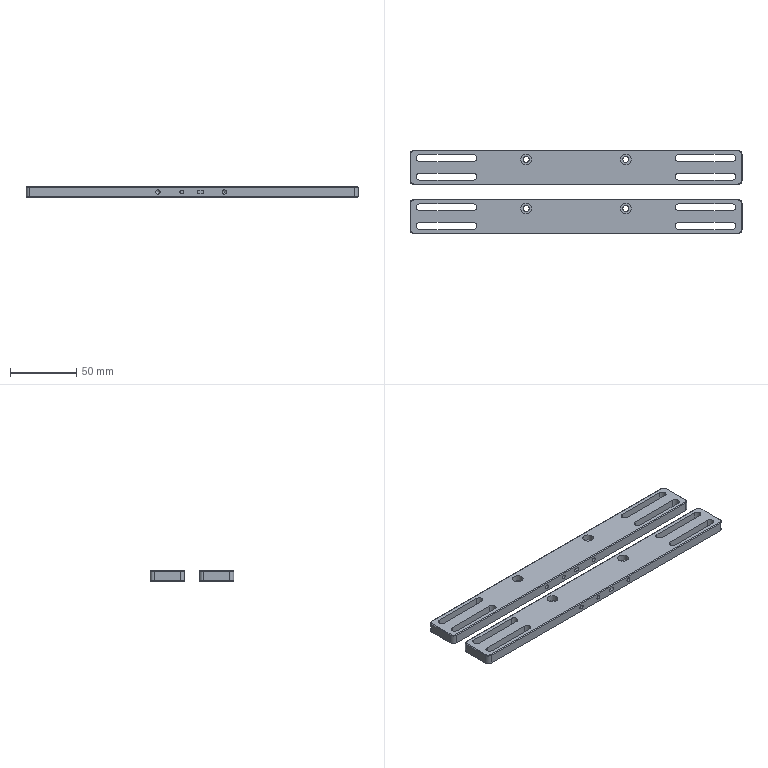NC program | NX | posted with a generic post | part box 250 x 63 x 8 mm
Lines 30 to 910 of 4328:
(ZLEVEL_PROFILE_COPY_COPY , TOOL : D2)
N52 T12 M6
N54 G54
N56 G17 G0 G90 X-7.077 Y0.4 B0. C0. S7500 M3
N58 G43 Z30. H12
N60 Z0.5
N62 G94 G1 X-7.191 Z0.494 F1000.
N64 X-7.207 Y0.396 Z0.493
N66 X-7.366 Y0.312 Z0.484
N68 X-7.496 Y0.108 Z0.471
N70 X-7.488 Y-0.134 Z0.458
N72 X-7.394 Y-0.287 Z0.449
N74 X-7.191 Y-0.4 Z0.437
N76 X-5.511 Z0.349
N78 X-5.323 Y-0.301 Z0.338
N80 X-5.209 Y-0.122 Z0.326
N82 X-5.195 Y0.057 Z0.317
N84 X-5.299 Y0.278 Z0.304
N86 X-5.511 Y0.4 Z0.291
N88 X-7.191 Z0.203
N90 X-7.207 Y0.396
N92 X-7.366 Y0.312 Z0.193
N94 X-7.496 Y0.108 Z0.18
N96 X-7.488 Y-0.134 Z0.168
N98 X-7.394 Y-0.287 Z0.158
N100 X-7.191 Y-0.4 Z0.146
N102 X-5.511 Z0.058
N104 X-5.323 Y-0.301 Z0.047
N106 X-5.209 Y-0.122 Z0.036
N108 X-5.195 Y0.057 Z0.026
N110 X-5.299 Y0.278 Z0.014
N112 X-5.511 Y0.4 Z0.001
N114 X-7.191 Z-0.087
N116 X-7.207 Y0.396 Z-0.088
N118 X-7.366 Y0.312 Z-0.098
N120 X-7.496 Y0.108 Z-0.11
N122 X-7.488 Y-0.134 Z-0.123
N124 X-7.394 Y-0.287 Z-0.132
N126 X-7.191 Y-0.4 Z-0.145
N128 X-7.101 Z-0.149
N130 X-5.601
N132 G3 X-5.201 Y0. R0.4
N134 X-5.601 Y0.4 R0.4
N136 G1 X-7.101
N138 G3 X-7.501 Y0. R0.4
N140 X-7.101 Y-0.4 R0.4
N142 G1 X-5.757 Z-0.198
N144 X-5.654 Y-0.399 Z-0.201
N146 X-5.555 Y-0.389 Z-0.205
N148 X-5.506 Y-0.381 Z-0.207
N150 X-5.454 Y-0.363 Z-0.209
N152 X-5.378 Y-0.321 Z-0.212
N154 X-5.344 Y-0.296 Z-0.214
N156 X-5.292 Y-0.244 Z-0.216
N158 X-5.251 Y-0.179 Z-0.219
N160 X-5.227 Y-0.116 Z-0.222
N162 X-5.214 Y-0.059 Z-0.224
N164 X-5.21 Y0.023 Z-0.227
N166 X-5.218 Y0.089 Z-0.229
N168 X-5.235 Y0.14 Z-0.231
N170 X-5.276 Y0.218 Z-0.235
N172 X-5.301 Y0.253 Z-0.236
N174 X-5.351 Y0.303 Z-0.239
N176 X-5.408 Y0.34 Z-0.241
N178 X-5.437 Y0.357 Z-0.243
N180 X-5.469 Y0.368 Z-0.244
N182 X-5.534 Y0.386 Z-0.246
N184 X-5.636 Y0.397 Z-0.25
N186 X-5.739 Y0.4 Z-0.254
N188 X-6.979 Z-0.299
N190 X-7.101
N192 G3 X-7.501 Y0. R0.4
N194 X-7.101 Y-0.4 R0.4
N196 G1 X-5.757 Z-0.347
N198 X-5.654 Y-0.399 Z-0.351
N200 X-5.555 Y-0.389 Z-0.354
N202 X-5.506 Y-0.381 Z-0.356
N204 X-5.454 Y-0.363 Z-0.358
N206 X-5.378 Y-0.321 Z-0.361
N208 X-5.344 Y-0.296 Z-0.363
N210 X-5.292 Y-0.244 Z-0.366
N212 X-5.251 Y-0.179 Z-0.368
N214 X-5.227 Y-0.116 Z-0.371
N216 X-5.214 Y-0.059 Z-0.373
N218 X-5.21 Y0.023 Z-0.376
N220 X-5.218 Y0.089 Z-0.379
N222 X-5.235 Y0.139 Z-0.381
N224 X-5.276 Y0.218 Z-0.384
N226 X-5.301 Y0.253 Z-0.385
N228 X-5.351 Y0.303 Z-0.388
N230 X-5.408 Y0.34 Z-0.391
N232 X-5.437 Y0.357 Z-0.392
N234 X-5.468 Y0.368 Z-0.393
N236 X-5.534 Y0.386 Z-0.396
N238 X-5.636 Y0.397 Z-0.399
N240 X-5.739 Y0.4 Z-0.403
N242 X-6.979 Z-0.448
N244 X-7.101
N246 G3 X-7.501 Y0. R0.4
N248 X-7.101 Y-0.4 R0.4
N250 G1 X-5.757 Z-0.496
N252 X-5.654 Y-0.399 Z-0.5
N254 X-5.555 Y-0.389 Z-0.504
N256 X-5.506 Y-0.381 Z-0.505
N258 X-5.454 Y-0.363 Z-0.507
N260 X-5.377 Y-0.322 Z-0.511
N262 X-5.344 Y-0.296 Z-0.512
N264 X-5.292 Y-0.244 Z-0.515
N266 X-5.251 Y-0.179 Z-0.518
N268 X-5.227 Y-0.116 Z-0.52
N270 X-5.214 Y-0.059 Z-0.522
N272 X-5.21 Y0.023 Z-0.525
N274 X-5.217 Y0.089 Z-0.528
N276 X-5.235 Y0.139 Z-0.53
N278 X-5.277 Y0.219 Z-0.533
N280 X-5.302 Y0.255 Z-0.535
N282 X-5.351 Y0.303 Z-0.537
N284 X-5.408 Y0.34 Z-0.54
N286 X-5.437 Y0.357 Z-0.541
N288 X-5.469 Y0.368 Z-0.542
N290 X-5.534 Y0.386 Z-0.545
N292 X-5.636 Y0.397 Z-0.549
N294 X-5.739 Y0.4 Z-0.552
N296 X-6.979 Z-0.597
N298 X-7.101
N300 G3 X-7.501 Y0. R0.4
N302 X-7.101 Y-0.4 R0.4
N304 G1 X-5.757 Z-0.646
N306 X-5.654 Y-0.399 Z-0.649
N308 X-5.555 Y-0.388 Z-0.653
N310 X-5.506 Y-0.381 Z-0.655
N312 X-5.454 Y-0.363 Z-0.657
N314 X-5.377 Y-0.322 Z-0.66
N316 X-5.344 Y-0.296 Z-0.661
N318 X-5.292 Y-0.244 Z-0.664
N320 X-5.251 Y-0.179 Z-0.667
N322 X-5.227 Y-0.116 Z-0.669
N324 X-5.214 Y-0.059 Z-0.672
N326 X-5.21 Y0.023 Z-0.675
N328 X-5.217 Y0.089 Z-0.677
N330 X-5.235 Y0.139 Z-0.679
N332 X-5.277 Y0.219 Z-0.682
N334 X-5.302 Y0.255 Z-0.684
N336 X-5.351 Y0.303 Z-0.687
N338 X-5.408 Y0.34 Z-0.689
N340 X-5.437 Y0.357 Z-0.69
N342 X-5.469 Y0.368 Z-0.692
N344 X-5.534 Y0.386 Z-0.694
N346 X-5.636 Y0.397 Z-0.698
N348 X-5.739 Y0.4 Z-0.701
N350 X-6.979 Z-0.746
N352 X-7.101
N354 G3 X-7.501 Y0. R0.4
N356 X-7.101 Y-0.4 R0.4
N358 G1 X-5.757 Z-0.795
N360 X-5.654 Y-0.399 Z-0.799
N362 X-5.555 Y-0.388 Z-0.802
N364 X-5.506 Y-0.381 Z-0.804
N366 X-5.454 Y-0.363 Z-0.806
N368 X-5.377 Y-0.322 Z-0.809
N370 X-5.344 Y-0.296 Z-0.811
N372 X-5.292 Y-0.244 Z-0.813
N374 X-5.251 Y-0.178 Z-0.816
N376 X-5.236 Y-0.143 Z-0.818
N378 X-5.227 Y-0.116 Z-0.819
N380 X-5.214 Y-0.059 Z-0.821
N382 X-5.21 Y0.023 Z-0.824
N384 X-5.217 Y0.09 Z-0.826
N386 X-5.235 Y0.139 Z-0.828
N388 X-5.277 Y0.219 Z-0.832
N390 X-5.302 Y0.255 Z-0.833
N392 X-5.351 Y0.303 Z-0.836
N394 X-5.408 Y0.34 Z-0.838
N396 X-5.437 Y0.357 Z-0.84
N398 X-5.469 Y0.368 Z-0.841
N400 X-5.534 Y0.386 Z-0.843
N402 X-5.636 Y0.397 Z-0.847
N404 X-5.739 Y0.4 Z-0.851
N406 X-6.979 Z-0.896
N408 X-7.101
N410 G3 X-7.501 Y0. R0.4
N412 X-7.101 Y-0.4 R0.4
N414 G1 X-5.757 Z-0.944
N416 X-5.654 Y-0.399 Z-0.948
N418 X-5.555 Y-0.388 Z-0.951
N420 X-5.506 Y-0.381 Z-0.953
N422 X-5.454 Y-0.363 Z-0.955
N424 X-5.377 Y-0.322 Z-0.958
N426 X-5.344 Y-0.296 Z-0.96
N428 X-5.292 Y-0.244 Z-0.963
N430 X-5.251 Y-0.178 Z-0.966
N432 X-5.236 Y-0.143 Z-0.967
N434 X-5.227 Y-0.116 Z-0.968
N436 X-5.214 Y-0.059 Z-0.97
N438 X-5.21 Y0.023 Z-0.973
N440 X-5.217 Y0.089 Z-0.976
N442 X-5.235 Y0.139 Z-0.978
N444 X-5.277 Y0.219 Z-0.981
N446 X-5.302 Y0.255 Z-0.983
N448 X-5.351 Y0.303 Z-0.985
N450 X-5.408 Y0.34 Z-0.988
N452 X-5.437 Y0.357 Z-0.989
N454 X-5.469 Y0.368 Z-0.99
N456 X-5.534 Y0.386 Z-0.993
N458 X-5.636 Y0.397 Z-0.996
N460 X-5.739 Y0.4 Z-1.
N462 X-6.979 Z-1.045
N464 X-7.101
N466 G3 X-7.501 Y0. R0.4
N468 X-7.101 Y-0.4 R0.4
N470 G1 X-5.757 Z-1.093
N472 X-5.654 Y-0.399 Z-1.097
N474 X-5.555 Y-0.388 Z-1.101
N476 X-5.506 Y-0.381 Z-1.102
N478 X-5.454 Y-0.363 Z-1.104
N480 X-5.377 Y-0.322 Z-1.108
N482 X-5.344 Y-0.296 Z-1.109
N484 X-5.292 Y-0.244 Z-1.112
N486 X-5.251 Y-0.178 Z-1.115
N488 X-5.236 Y-0.143 Z-1.116
N490 X-5.227 Y-0.116 Z-1.117
N492 X-5.214 Y-0.059 Z-1.119
N494 X-5.21 Y0.023 Z-1.122
N496 X-5.217 Y0.089 Z-1.125
N498 X-5.235 Y0.139 Z-1.127
N500 X-5.277 Y0.219 Z-1.13
N502 X-5.302 Y0.255 Z-1.132
N504 X-5.351 Y0.303 Z-1.134
N506 X-5.408 Y0.34 Z-1.137
N508 X-5.437 Y0.357 Z-1.138
N510 X-5.469 Y0.368 Z-1.139
N512 X-5.534 Y0.386 Z-1.142
N514 X-5.636 Y0.397 Z-1.146
N516 X-5.739 Y0.4 Z-1.149
N518 X-6.979 Z-1.194
N520 X-7.101
N522 G3 X-7.501 Y0. R0.4
N524 X-7.101 Y-0.4 R0.4
N526 G1 X-5.757 Z-1.243
N528 X-5.654 Y-0.399 Z-1.246
N530 X-5.555 Y-0.388 Z-1.25
N532 X-5.506 Y-0.381 Z-1.252
N534 X-5.454 Y-0.363 Z-1.254
N536 X-5.377 Y-0.322 Z-1.257
N538 X-5.344 Y-0.296 Z-1.258
N540 X-5.292 Y-0.244 Z-1.261
N542 X-5.251 Y-0.178 Z-1.264
N544 X-5.236 Y-0.143 Z-1.265
N546 X-5.227 Y-0.116 Z-1.267
N548 X-5.214 Y-0.059 Z-1.269
N550 X-5.21 Y0.023 Z-1.272
N552 X-5.217 Y0.089 Z-1.274
N554 X-5.236 Y0.139 Z-1.276
N556 X-5.277 Y0.219 Z-1.279
N558 X-5.302 Y0.255 Z-1.281
N560 X-5.351 Y0.303 Z-1.284
N562 X-5.408 Y0.34 Z-1.286
N564 X-5.437 Y0.357 Z-1.287
N566 X-5.469 Y0.368 Z-1.289
N568 X-5.534 Y0.386 Z-1.291
N570 X-5.636 Y0.397 Z-1.295
N572 X-5.739 Y0.4 Z-1.299
N574 X-6.979 Z-1.343
N576 X-7.101
N578 G3 X-7.501 Y0. R0.4
N580 X-7.101 Y-0.4 R0.4
N582 G1 X-5.757 Z-1.392
N584 X-5.654 Y-0.399 Z-1.396
N586 X-5.555 Y-0.388 Z-1.399
N588 X-5.506 Y-0.381 Z-1.401
N590 X-5.454 Y-0.363 Z-1.403
N592 X-5.377 Y-0.322 Z-1.406
N594 X-5.344 Y-0.296 Z-1.408
N596 X-5.292 Y-0.244 Z-1.41
N598 X-5.251 Y-0.178 Z-1.413
N600 X-5.236 Y-0.143 Z-1.415
N602 X-5.227 Y-0.116 Z-1.416
N604 X-5.214 Y-0.059 Z-1.418
N606 X-5.21 Y0.023 Z-1.421
N608 X-5.218 Y0.089 Z-1.423
N610 X-5.236 Y0.139 Z-1.425
N612 X-5.276 Y0.219 Z-1.429
N614 X-5.302 Y0.255 Z-1.43
N616 X-5.351 Y0.303 Z-1.433
N618 X-5.408 Y0.34 Z-1.435
N620 X-5.437 Y0.357 Z-1.437
N622 X-5.469 Y0.368 Z-1.438
N624 X-5.534 Y0.386 Z-1.44
N626 X-5.636 Y0.397 Z-1.444
N628 X-5.739 Y0.4 Z-1.448
N630 X-6.979 Z-1.493
N632 X-7.101
N634 G3 X-7.501 Y0. R0.4
N636 X-7.101 Y-0.4 R0.4
N638 G1 X-5.757 Z-1.541
N640 X-5.654 Y-0.399 Z-1.545
N642 X-5.555 Y-0.388 Z-1.548
N644 X-5.506 Y-0.381 Z-1.55
N646 X-5.454 Y-0.363 Z-1.552
N648 X-5.377 Y-0.322 Z-1.555
N650 X-5.344 Y-0.296 Z-1.557
N652 X-5.292 Y-0.244 Z-1.56
N654 X-5.251 Y-0.178 Z-1.563
N656 X-5.236 Y-0.143 Z-1.564
N658 X-5.227 Y-0.116 Z-1.565
N660 X-5.214 Y-0.059 Z-1.567
N662 X-5.21 Y0.023 Z-1.57
N664 X-5.218 Y0.089 Z-1.573
N666 X-5.236 Y0.139 Z-1.575
N668 X-5.276 Y0.219 Z-1.578
N670 X-5.302 Y0.255 Z-1.58
N672 X-5.351 Y0.303 Z-1.582
N674 X-5.408 Y0.34 Z-1.585
N676 X-5.437 Y0.357 Z-1.586
N678 X-5.469 Y0.368 Z-1.587
N680 X-5.534 Y0.386 Z-1.59
N682 X-5.636 Y0.397 Z-1.593
N684 X-5.739 Y0.4 Z-1.597
N686 X-6.979 Z-1.642
N688 X-7.101
N690 G3 X-7.501 Y0. R0.4
N692 X-7.101 Y-0.4 R0.4
N694 G1 X-5.757 Z-1.69
N696 X-5.654 Y-0.399 Z-1.694
N698 X-5.555 Y-0.388 Z-1.698
N700 X-5.506 Y-0.381 Z-1.699
N702 X-5.454 Y-0.363 Z-1.701
N704 X-5.377 Y-0.322 Z-1.705
N706 X-5.344 Y-0.296 Z-1.706
N708 X-5.292 Y-0.244 Z-1.709
N710 X-5.251 Y-0.178 Z-1.712
N712 X-5.237 Y-0.143 Z-1.713
N714 X-5.227 Y-0.116 Z-1.714
N716 X-5.214 Y-0.059 Z-1.716
N718 X-5.21 Y0.023 Z-1.719
N720 X-5.218 Y0.089 Z-1.722
N722 X-5.236 Y0.139 Z-1.724
N724 X-5.276 Y0.219 Z-1.727
N726 X-5.302 Y0.254 Z-1.729
N728 X-5.351 Y0.303 Z-1.731
N730 X-5.408 Y0.34 Z-1.734
N732 X-5.437 Y0.357 Z-1.735
N734 X-5.469 Y0.368 Z-1.736
N736 X-5.534 Y0.386 Z-1.739
N738 X-5.636 Y0.397 Z-1.743
N740 X-5.739 Y0.4 Z-1.746
N742 X-6.979 Z-1.791
N744 X-7.101
N746 G3 X-7.501 Y0. R0.4
N748 X-7.101 Y-0.4 R0.4
N750 G1 X-5.757 Z-1.84
N752 X-5.654 Y-0.399 Z-1.843
N754 X-5.555 Y-0.388 Z-1.847
N756 X-5.506 Y-0.381 Z-1.849
N758 X-5.454 Y-0.363 Z-1.851
N760 X-5.377 Y-0.322 Z-1.854
N762 X-5.344 Y-0.296 Z-1.855
N764 X-5.292 Y-0.244 Z-1.858
N766 X-5.251 Y-0.178 Z-1.861
N768 X-5.237 Y-0.143 Z-1.862
N770 X-5.227 Y-0.116 Z-1.864
N772 X-5.214 Y-0.059 Z-1.866
N774 X-5.21 Y0.023 Z-1.869
N776 X-5.218 Y0.089 Z-1.871
N778 X-5.236 Y0.139 Z-1.873
N780 X-5.276 Y0.219 Z-1.876
N782 X-5.302 Y0.254 Z-1.878
N784 X-5.351 Y0.303 Z-1.881
N786 X-5.408 Y0.34 Z-1.883
N788 X-5.437 Y0.357 Z-1.884
N790 X-5.469 Y0.368 Z-1.886
N792 X-5.534 Y0.386 Z-1.888
N794 X-5.636 Y0.397 Z-1.892
N796 X-5.739 Y0.4 Z-1.896
N798 X-6.979 Z-1.94
N800 X-7.101
N802 G3 X-7.501 Y0. R0.4
N804 X-7.101 Y-0.4 R0.4
N806 G1 X-5.757 Z-1.989
N808 X-5.654 Y-0.399 Z-1.993
N810 X-5.555 Y-0.388 Z-1.996
N812 X-5.506 Y-0.381 Z-1.998
N814 X-5.454 Y-0.363 Z-2.
N816 X-5.378 Y-0.322 Z-2.003
N818 X-5.344 Y-0.296 Z-2.005
N820 X-5.292 Y-0.244 Z-2.007
N822 X-5.251 Y-0.178 Z-2.01
N824 X-5.237 Y-0.143 Z-2.012
N826 X-5.227 Y-0.116 Z-2.013
N828 X-5.214 Y-0.059 Z-2.015
N830 X-5.21 Y0.023 Z-2.018
N832 X-5.218 Y0.089 Z-2.02
N834 X-5.236 Y0.139 Z-2.022
N836 X-5.276 Y0.219 Z-2.026
N838 X-5.302 Y0.254 Z-2.027
N840 X-5.351 Y0.303 Z-2.03
N842 X-5.408 Y0.34 Z-2.032
N844 X-5.437 Y0.357 Z-2.034
N846 X-5.469 Y0.368 Z-2.035
N848 X-5.534 Y0.386 Z-2.037
N850 X-5.636 Y0.397 Z-2.041
N852 X-5.739 Y0.4 Z-2.045
N854 X-6.979 Z-2.09
N856 X-7.101
N858 G3 X-7.501 Y0. R0.4
N860 X-7.101 Y-0.4 R0.4
N862 G1 X-5.757 Z-2.138
N864 X-5.654 Y-0.399 Z-2.142
N866 X-5.555 Y-0.388 Z-2.145
N868 X-5.506 Y-0.381 Z-2.147
N870 X-5.454 Y-0.363 Z-2.149
N872 X-5.378 Y-0.322 Z-2.152
N874 X-5.344 Y-0.296 Z-2.154
N876 X-5.292 Y-0.244 Z-2.157
N878 X-5.251 Y-0.178 Z-2.16
N880 X-5.237 Y-0.143 Z-2.161
N882 X-5.227 Y-0.116 Z-2.162
N884 X-5.214 Y-0.059 Z-2.164
N886 X-5.21 Y0.023 Z-2.167
N888 X-5.218 Y0.089 Z-2.17
N890 X-5.236 Y0.139 Z-2.172
N892 X-5.276 Y0.219 Z-2.175
N894 X-5.302 Y0.254 Z-2.177
N896 X-5.351 Y0.303 Z-2.179
N898 X-5.408 Y0.34 Z-2.182
N900 X-5.437 Y0.357 Z-2.183
N902 X-5.469 Y0.368 Z-2.184
N904 X-5.534 Y0.386 Z-2.187
N906 X-5.636 Y0.397 Z-2.19
N908 X-5.739 Y0.4 Z-2.194
N910 X-6.979 Z-2.239
N912 X-7.101
N914 G3 X-7.501 Y0. R0.4
N916 X-7.101 Y-0.4 R0.4
N918 G1 X-5.757 Z-2.287
N920 X-5.654 Y-0.399 Z-2.291
N922 X-5.555 Y-0.388 Z-2.295
N924 X-5.506 Y-0.381 Z-2.296
N926 X-5.454 Y-0.363 Z-2.299
N928 X-5.378 Y-0.322 Z-2.302
N930 X-5.344 Y-0.296 Z-2.303
N932 X-5.292 Y-0.244 Z-2.306
N934 X-5.251 Y-0.178 Z-2.309
N936 X-5.237 Y-0.143 Z-2.31
N938 X-5.227 Y-0.116 Z-2.311
N940 X-5.214 Y-0.059 Z-2.313
N942 X-5.21 Y0.023 Z-2.316
N944 X-5.218 Y0.089 Z-2.319
N946 X-5.236 Y0.139 Z-2.321
N948 X-5.276 Y0.219 Z-2.324
N950 X-5.302 Y0.254 Z-2.326
N952 X-5.351 Y0.303 Z-2.328
N954 X-5.408 Y0.34 Z-2.331
N956 X-5.437 Y0.357 Z-2.332
N958 X-5.468 Y0.368 Z-2.333
N960 X-5.534 Y0.386 Z-2.336
N962 X-5.636 Y0.397 Z-2.34
N964 X-5.739 Y0.4 Z-2.343
N966 X-6.979 Z-2.388
N968 X-7.101
N970 G3 X-7.501 Y0. R0.4
N972 X-7.101 Y-0.4 R0.4
N974 G1 X-5.757 Z-2.437
N976 X-5.654 Y-0.399 Z-2.44
N978 X-5.555 Y-0.388 Z-2.444
N980 X-5.506 Y-0.381 Z-2.446
N982 X-5.454 Y-0.363 Z-2.448
N984 X-5.378 Y-0.322 Z-2.451
N986 X-5.344 Y-0.296 Z-2.452
N988 X-5.292 Y-0.244 Z-2.455
N990 X-5.251 Y-0.178 Z-2.458
N992 X-5.237 Y-0.143 Z-2.459
N994 X-5.227 Y-0.116 Z-2.461
N996 X-5.214 Y-0.059 Z-2.463
N998 X-5.21 Y0.023 Z-2.466
N1000 X-5.218 Y0.089 Z-2.468
N1002 X-5.236 Y0.139 Z-2.47
N1004 X-5.276 Y0.219 Z-2.473
N1006 X-5.302 Y0.254 Z-2.475
N1008 X-5.351 Y0.303 Z-2.478
N1010 X-5.408 Y0.34 Z-2.48
N1012 X-5.437 Y0.357 Z-2.481
N1014 X-5.468 Y0.368 Z-2.483
N1016 X-5.534 Y0.386 Z-2.485
N1018 X-5.636 Y0.397 Z-2.489
N1020 X-5.739 Y0.4 Z-2.493
N1022 X-6.979 Z-2.537
N1024 X-7.101
N1026 G3 X-7.501 Y0. R0.4
N1028 X-7.101 Y-0.4 R0.4
N1030 G1 X-5.757 Z-2.586
N1032 X-5.654 Y-0.399 Z-2.59
N1034 X-5.555 Y-0.388 Z-2.593
N1036 X-5.506 Y-0.381 Z-2.595
N1038 X-5.454 Y-0.363 Z-2.597
N1040 X-5.378 Y-0.322 Z-2.6
N1042 X-5.344 Y-0.296 Z-2.602
N1044 X-5.292 Y-0.244 Z-2.604
N1046 X-5.252 Y-0.178 Z-2.607
N1048 X-5.237 Y-0.143 Z-2.609
N1050 X-5.227 Y-0.116 Z-2.61
N1052 X-5.214 Y-0.059 Z-2.612
N1054 X-5.21 Y0.023 Z-2.615
N1056 X-5.218 Y0.089 Z-2.617
N1058 X-5.236 Y0.139 Z-2.619
N1060 X-5.276 Y0.219 Z-2.623
N1062 X-5.302 Y0.254 Z-2.624
N1064 X-5.351 Y0.303 Z-2.627
N1066 X-5.408 Y0.34 Z-2.629
N1068 X-5.437 Y0.357 Z-2.631
N1070 X-5.468 Y0.368 Z-2.632
N1072 X-5.534 Y0.386 Z-2.634
N1074 X-5.636 Y0.397 Z-2.638
N1076 X-5.739 Y0.4 Z-2.642
N1078 X-6.979 Z-2.687
N1080 X-7.101
N1082 G3 X-7.501 Y0. R0.4
N1084 X-7.101 Y-0.4 R0.4
N1086 G1 X-5.757 Z-2.735
N1088 X-5.654 Y-0.399 Z-2.739
N1090 X-5.555 Y-0.388 Z-2.742
N1092 X-5.506 Y-0.381 Z-2.744
N1094 X-5.454 Y-0.363 Z-2.746
N1096 X-5.378 Y-0.322 Z-2.749
N1098 X-5.344 Y-0.296 Z-2.751
N1100 X-5.292 Y-0.244 Z-2.754
N1102 X-5.252 Y-0.178 Z-2.757
N1104 X-5.237 Y-0.143 Z-2.758
N1106 X-5.227 Y-0.116 Z-2.759
N1108 X-5.214 Y-0.059 Z-2.761
N1110 X-5.21 Y0.023 Z-2.764
N1112 X-5.218 Y0.089 Z-2.767
N1114 X-5.236 Y0.139 Z-2.769
N1116 X-5.276 Y0.219 Z-2.772
N1118 X-5.302 Y0.254 Z-2.774
N1120 X-5.351 Y0.303 Z-2.776
N1122 X-5.408 Y0.34 Z-2.779
N1124 X-5.437 Y0.357 Z-2.78
N1126 X-5.468 Y0.368 Z-2.781
N1128 X-5.534 Y0.386 Z-2.784
N1130 X-5.636 Y0.397 Z-2.787
N1132 X-5.739 Y0.4 Z-2.791
N1134 X-6.979 Z-2.836
N1136 X-7.101
N1138 G3 X-7.501 Y0. R0.4
N1140 X-7.101 Y-0.4 R0.4
N1142 G1 X-5.757 Z-2.884
N1144 X-5.654 Y-0.399 Z-2.888
N1146 X-5.555 Y-0.388 Z-2.892
N1148 X-5.506 Y-0.381 Z-2.893
N1150 X-5.454 Y-0.363 Z-2.896
N1152 X-5.378 Y-0.322 Z-2.899
N1154 X-5.344 Y-0.296 Z-2.9
N1156 X-5.292 Y-0.244 Z-2.903
N1158 X-5.252 Y-0.178 Z-2.906
N1160 X-5.237 Y-0.143 Z-2.907
N1162 X-5.227 Y-0.116 Z-2.908
N1164 X-5.214 Y-0.059 Z-2.91
N1166 X-5.21 Y0.023 Z-2.913
N1168 X-5.218 Y0.089 Z-2.916
N1170 X-5.236 Y0.139 Z-2.918
N1172 X-5.276 Y0.219 Z-2.921
N1174 X-5.302 Y0.254 Z-2.923
N1176 X-5.351 Y0.303 Z-2.925
N1178 X-5.408 Y0.34 Z-2.928
N1180 X-5.437 Y0.357 Z-2.929
N1182 X-5.468 Y0.368 Z-2.93
N1184 X-5.534 Y0.386 Z-2.933
N1186 X-5.636 Y0.397 Z-2.937
N1188 X-5.739 Y0.4 Z-2.94
N1190 X-6.979 Z-2.985
N1192 X-7.101
N1194 G3 X-7.501 Y0. R0.4
N1196 X-7.101 Y-0.4 R0.4
N1198 G1 X-5.757 Z-3.034
N1200 X-5.654 Y-0.399 Z-3.037
N1202 X-5.555 Y-0.388 Z-3.041
N1204 X-5.506 Y-0.381 Z-3.043
N1206 X-5.454 Y-0.363 Z-3.045
N1208 X-5.377 Y-0.321 Z-3.048
N1210 X-5.344 Y-0.295 Z-3.05
N1212 X-5.292 Y-0.244 Z-3.052
N1214 X-5.251 Y-0.178 Z-3.055
N1216 X-5.227 Y-0.116 Z-3.058
N1218 X-5.214 Y-0.059 Z-3.06
N1220 X-5.21 Y0.023 Z-3.063
N1222 X-5.218 Y0.089 Z-3.065
N1224 X-5.236 Y0.139 Z-3.067
N1226 X-5.276 Y0.219 Z-3.07
N1228 X-5.302 Y0.254 Z-3.072
N1230 X-5.351 Y0.303 Z-3.075
N1232 X-5.408 Y0.34 Z-3.077
N1234 X-5.437 Y0.357 Z-3.078
N1236 X-5.468 Y0.368 Z-3.08
N1238 X-5.534 Y0.386 Z-3.082
N1240 X-5.636 Y0.397 Z-3.086
N1242 X-5.739 Y0.4 Z-3.09
N1244 X-6.979 Z-3.134
N1246 X-7.101
N1248 G3 X-7.501 Y0. R0.4
N1250 X-7.101 Y-0.4 R0.4
N1252 G1 X-5.757 Z-3.183
N1254 X-5.654 Y-0.399 Z-3.187
N1256 X-5.555 Y-0.388 Z-3.19
N1258 X-5.506 Y-0.381 Z-3.192
N1260 X-5.454 Y-0.363 Z-3.194
N1262 X-5.377 Y-0.321 Z-3.197
N1264 X-5.344 Y-0.295 Z-3.199
N1266 X-5.292 Y-0.244 Z-3.201
N1268 X-5.251 Y-0.178 Z-3.204
N1270 X-5.227 Y-0.116 Z-3.207
N1272 X-5.214 Y-0.059 Z-3.209
N1274 X-5.21 Y0.023 Z-3.212
N1276 X-5.218 Y0.089 Z-3.214
N1278 X-5.236 Y0.139 Z-3.216
N1280 X-5.276 Y0.219 Z-3.22
N1282 X-5.302 Y0.254 Z-3.221
N1284 X-5.351 Y0.303 Z-3.224
N1286 X-5.408 Y0.341 Z-3.226
N1288 X-5.438 Y0.357 Z-3.228
N1290 X-5.469 Y0.368 Z-3.229
N1292 X-5.534 Y0.386 Z-3.231
N1294 X-5.636 Y0.397 Z-3.235
N1296 X-5.739 Y0.4 Z-3.239
N1298 X-6.979 Z-3.284
N1300 X-7.101
N1302 G3 X-7.501 Y0. R0.4
N1304 X-7.101 Y-0.4 R0.4
N1306 G1 X-5.757 Z-3.332
N1308 X-5.654 Y-0.399 Z-3.336
N1310 X-5.555 Y-0.388 Z-3.339
N1312 X-5.506 Y-0.381 Z-3.341
N1314 X-5.454 Y-0.363 Z-3.343
N1316 X-5.377 Y-0.321 Z-3.346
N1318 X-5.344 Y-0.295 Z-3.348
N1320 X-5.292 Y-0.244 Z-3.351
N1322 X-5.251 Y-0.178 Z-3.354
N1324 X-5.227 Y-0.116 Z-3.356
N1326 X-5.214 Y-0.059 Z-3.358
N1328 X-5.21 Y0.023 Z-3.361
N1330 X-5.218 Y0.089 Z-3.364
N1332 X-5.236 Y0.139 Z-3.366
N1334 X-5.276 Y0.219 Z-3.369
N1336 X-5.302 Y0.254 Z-3.371
N1338 X-5.351 Y0.303 Z-3.373
N1340 X-5.408 Y0.341 Z-3.376
N1342 X-5.438 Y0.357 Z-3.377
N1344 X-5.469 Y0.368 Z-3.378
N1346 X-5.534 Y0.386 Z-3.381
N1348 X-5.636 Y0.397 Z-3.384
N1350 X-5.739 Y0.4 Z-3.388
N1352 X-6.979 Z-3.433
N1354 X-7.101
N1356 G3 X-7.501 Y0. R0.4
N1358 X-7.101 Y-0.4 R0.4
N1360 G1 X-5.757 Z-3.481
N1362 X-5.654 Y-0.399 Z-3.485
N1364 X-5.555 Y-0.388 Z-3.489
N1366 X-5.506 Y-0.381 Z-3.491
N1368 X-5.454 Y-0.363 Z-3.493
N1370 X-5.377 Y-0.321 Z-3.496
N1372 X-5.344 Y-0.295 Z-3.497
N1374 X-5.292 Y-0.244 Z-3.5
N1376 X-5.251 Y-0.178 Z-3.503
N1378 X-5.227 Y-0.116 Z-3.505
N1380 X-5.214 Y-0.059 Z-3.507
N1382 X-5.21 Y0.023 Z-3.51
N1384 X-5.218 Y0.089 Z-3.513
N1386 X-5.236 Y0.139 Z-3.515
N1388 X-5.276 Y0.219 Z-3.518
N1390 X-5.302 Y0.254 Z-3.52
N1392 X-5.351 Y0.303 Z-3.522
N1394 X-5.408 Y0.341 Z-3.525
N1396 X-5.438 Y0.357 Z-3.526
N1398 X-5.469 Y0.368 Z-3.527
N1400 X-5.534 Y0.386 Z-3.53
N1402 X-5.636 Y0.397 Z-3.534
N1404 X-5.739 Y0.4 Z-3.537
N1406 X-6.979 Z-3.582
N1408 X-7.101
N1410 G3 X-7.501 Y0. R0.4
N1412 X-7.101 Y-0.4 R0.4
N1414 G1 X-5.757 Z-3.631
N1416 X-5.654 Y-0.399 Z-3.634
N1418 X-5.555 Y-0.388 Z-3.638
N1420 X-5.506 Y-0.381 Z-3.64
N1422 X-5.454 Y-0.363 Z-3.642
N1424 X-5.377 Y-0.321 Z-3.645
N1426 X-5.344 Y-0.295 Z-3.647
N1428 X-5.292 Y-0.244 Z-3.649
N1430 X-5.251 Y-0.178 Z-3.652
N1432 X-5.227 Y-0.116 Z-3.655
N1434 X-5.215 Y-0.059 Z-3.657
N1436 X-5.21 Y0.023 Z-3.66
N1438 X-5.218 Y0.089 Z-3.662
N1440 X-5.236 Y0.139 Z-3.664
N1442 X-5.276 Y0.219 Z-3.667
N1444 X-5.302 Y0.254 Z-3.669
N1446 X-5.351 Y0.303 Z-3.672
N1448 X-5.408 Y0.341 Z-3.674
N1450 X-5.438 Y0.357 Z-3.675
N1452 X-5.469 Y0.368 Z-3.677
N1454 X-5.534 Y0.386 Z-3.679
N1456 X-5.636 Y0.397 Z-3.683
N1458 X-5.739 Y0.4 Z-3.687
N1460 X-6.979 Z-3.731
N1462 X-7.101
N1464 G3 X-7.501 Y0. R0.4
N1466 X-7.101 Y-0.4 R0.4
N1468 G1 X-5.757 Z-3.78
N1470 X-5.654 Y-0.399 Z-3.784
N1472 X-5.555 Y-0.388 Z-3.787
N1474 X-5.506 Y-0.381 Z-3.789
N1476 X-5.454 Y-0.363 Z-3.791
N1478 X-5.377 Y-0.321 Z-3.794
N1480 X-5.344 Y-0.295 Z-3.796
N1482 X-5.292 Y-0.244 Z-3.799
N1484 X-5.251 Y-0.178 Z-3.801
N1486 X-5.227 Y-0.116 Z-3.804
N1488 X-5.215 Y-0.059 Z-3.806
N1490 X-5.21 Y0.023 Z-3.809
N1492 X-5.218 Y0.089 Z-3.811
N1494 X-5.236 Y0.139 Z-3.813
N1496 X-5.276 Y0.219 Z-3.817
N1498 X-5.302 Y0.254 Z-3.818
N1500 X-5.351 Y0.303 Z-3.821
N1502 X-5.408 Y0.341 Z-3.823
N1504 X-5.438 Y0.357 Z-3.825
N1506 X-5.469 Y0.368 Z-3.826
N1508 X-5.534 Y0.386 Z-3.828
N1510 X-5.636 Y0.397 Z-3.832
N1512 X-5.739 Y0.4 Z-3.836
N1514 X-6.979 Z-3.881
N1516 X-7.101
N1518 G3 X-7.501 Y0. R0.4
N1520 X-7.101 Y-0.4 R0.4
N1522 G1 X-5.757 Z-3.929
N1524 X-5.654 Y-0.399 Z-3.933
N1526 X-5.555 Y-0.388 Z-3.936
N1528 X-5.506 Y-0.381 Z-3.938
N1530 X-5.454 Y-0.363 Z-3.94
N1532 X-5.377 Y-0.321 Z-3.943
N1534 X-5.344 Y-0.295 Z-3.945
N1536 X-5.292 Y-0.244 Z-3.948
N1538 X-5.251 Y-0.178 Z-3.951
N1540 X-5.228 Y-0.116 Z-3.953
N1542 X-5.215 Y-0.059 Z-3.955
N1544 X-5.21 Y0.023 Z-3.958
N1546 X-5.218 Y0.089 Z-3.961
N1548 X-5.236 Y0.139 Z-3.963
N1550 X-5.276 Y0.219 Z-3.966
N1552 X-5.302 Y0.253 Z-3.968
N1554 X-5.351 Y0.303 Z-3.97
N1556 X-5.408 Y0.341 Z-3.973
N1558 X-5.438 Y0.357 Z-3.974
N1560 X-5.469 Y0.368 Z-3.975
N1562 X-5.534 Y0.386 Z-3.978
N1564 X-5.636 Y0.397 Z-3.981
N1566 X-5.739 Y0.4 Z-3.985
N1568 X-6.979 Z-4.03
N1570 X-7.101
N1572 G3 X-7.501 Y0. R0.4
N1574 X-7.101 Y-0.4 R0.4
N1576 G1 X-5.757 Z-4.078
N1578 X-5.654 Y-0.399 Z-4.082
N1580 X-5.555 Y-0.388 Z-4.086
N1582 X-5.506 Y-0.381 Z-4.088
N1584 X-5.454 Y-0.363 Z-4.09
N1586 X-5.378 Y-0.321 Z-4.093
N1588 X-5.344 Y-0.295 Z-4.094
N1590 X-5.292 Y-0.244 Z-4.097
N1592 X-5.251 Y-0.178 Z-4.1
N1594 X-5.228 Y-0.116 Z-4.102
N1596 X-5.215 Y-0.059 Z-4.104
N1598 X-5.21 Y0.023 Z-4.107
N1600 X-5.218 Y0.089 Z-4.11
N1602 X-5.236 Y0.139 Z-4.112
N1604 X-5.276 Y0.219 Z-4.115
N1606 X-5.302 Y0.253 Z-4.117
N1608 X-5.351 Y0.303 Z-4.119
N1610 X-5.408 Y0.341 Z-4.122
N1612 X-5.438 Y0.357 Z-4.123
N1614 X-5.469 Y0.368 Z-4.124
N1616 X-5.534 Y0.386 Z-4.127
N1618 X-5.636 Y0.397 Z-4.131
N1620 X-5.739 Y0.4 Z-4.134
N1622 X-6.979 Z-4.179
N1624 X-7.101
N1626 G3 X-7.501 Y0. R0.4
N1628 X-7.101 Y-0.4 R0.4
N1630 G1 X-5.757 Z-4.228
N1632 X-5.654 Y-0.399 Z-4.231
N1634 X-5.506 Y-0.381 Z-4.237
N1636 X-5.454 Y-0.363 Z-4.239
N1638 X-5.378 Y-0.322 Z-4.242
N1640 X-5.345 Y-0.296 Z-4.244
N1642 X-5.292 Y-0.244 Z-4.246
N1644 X-5.251 Y-0.179 Z-4.249
N1646 X-5.228 Y-0.116 Z-4.252
N1648 X-5.215 Y-0.059 Z-4.254
N1650 X-5.21 Y0.023 Z-4.257
N1652 X-5.218 Y0.089 Z-4.259
N1654 X-5.236 Y0.139 Z-4.261
N1656 X-5.276 Y0.218 Z-4.264
N1658 X-5.302 Y0.253 Z-4.266
N1660 X-5.351 Y0.303 Z-4.269
N1662 X-5.408 Y0.341 Z-4.271
N1664 X-5.438 Y0.357 Z-4.272
N1666 X-5.469 Y0.368 Z-4.274
N1668 X-5.534 Y0.386 Z-4.276
N1670 X-5.636 Y0.397 Z-4.28
N1672 X-5.739 Y0.4 Z-4.284
N1674 X-6.979 Z-4.328
N1676 X-7.101
N1678 G3 X-7.501 Y0. R0.4
N1680 X-7.101 Y-0.4 R0.4
N1682 G1 X-5.757 Z-4.377
N1684 X-5.654 Y-0.399 Z-4.381
N1686 X-5.505 Y-0.381 Z-4.386
N1688 X-5.454 Y-0.363 Z-4.388
N1690 X-5.378 Y-0.322 Z-4.391
N1692 X-5.345 Y-0.296 Z-4.393
N1694 X-5.292 Y-0.244 Z-4.396
N1696 X-5.251 Y-0.179 Z-4.398
N1698 X-5.228 Y-0.116 Z-4.401
N1700 X-5.215 Y-0.059 Z-4.403
N1702 X-5.21 Y0.023 Z-4.406
N1704 X-5.218 Y0.089 Z-4.408
N1706 X-5.236 Y0.139 Z-4.41
N1708 X-5.276 Y0.218 Z-4.414
N1710 X-5.302 Y0.253 Z-4.415
N1712 X-5.351 Y0.303 Z-4.418
N1714 X-5.408 Y0.341 Z-4.42
N1716 X-5.438 Y0.357 Z-4.422
N1718 X-5.469 Y0.368 Z-4.423
N1720 X-5.534 Y0.386 Z-4.425
N1722 X-5.636 Y0.397 Z-4.429
N1724 X-5.739 Y0.4 Z-4.433
N1726 X-6.979 Z-4.478
N1728 X-7.101
N1730 G3 X-7.501 Y0. R0.4
N1732 X-7.101 Y-0.4 R0.4
N1734 G1 X-5.757 Z-4.526
N1736 X-5.654 Y-0.399 Z-4.53
N1738 X-5.505 Y-0.381 Z-4.535
N1740 X-5.454 Y-0.363 Z-4.537
N1742 X-5.378 Y-0.322 Z-4.54
N1744 X-5.345 Y-0.296 Z-4.542
N1746 X-5.292 Y-0.244 Z-4.545
N1748 X-5.251 Y-0.179 Z-4.548
N1750 X-5.228 Y-0.116 Z-4.55
N1752 X-5.215 Y-0.059 Z-4.552
N1754 X-5.21 Y0.023 Z-4.555
N1756 X-5.218 Y0.089 Z-4.558
N1758 X-5.236 Y0.139 Z-4.56
N1760 X-5.276 Y0.218 Z-4.563
N1762 X-5.302 Y0.253 Z-4.565
N1764 X-5.351 Y0.303 Z-4.567
N1766 X-5.408 Y0.341 Z-4.57
N1768 X-5.438 Y0.357 Z-4.571
N1770 X-5.469 Y0.368 Z-4.572
N1772 X-5.534 Y0.386 Z-4.575
N1774 X-5.636 Y0.397 Z-4.578
N1776 X-5.739 Y0.4 Z-4.582
N1778 X-6.979 Z-4.627
N1780 X-7.101
N1782 G3 X-7.501 Y0. R0.4
N1784 X-7.101 Y-0.4 R0.4
N1786 G1 X-5.757 Z-4.675
N1788 X-5.654 Y-0.399 Z-4.679
N1790 X-5.505 Y-0.381 Z-4.685
N1792 X-5.454 Y-0.363 Z-4.687
N1794 X-5.378 Y-0.322 Z-4.69
N1796 X-5.345 Y-0.296 Z-4.691
N1798 X-5.292 Y-0.244 Z-4.694
N1800 X-5.251 Y-0.179 Z-4.697
N1802 X-5.228 Y-0.116 Z-4.699
N1804 X-5.215 Y-0.059 Z-4.701
N1806 X-5.21 Y0.023 Z-4.704